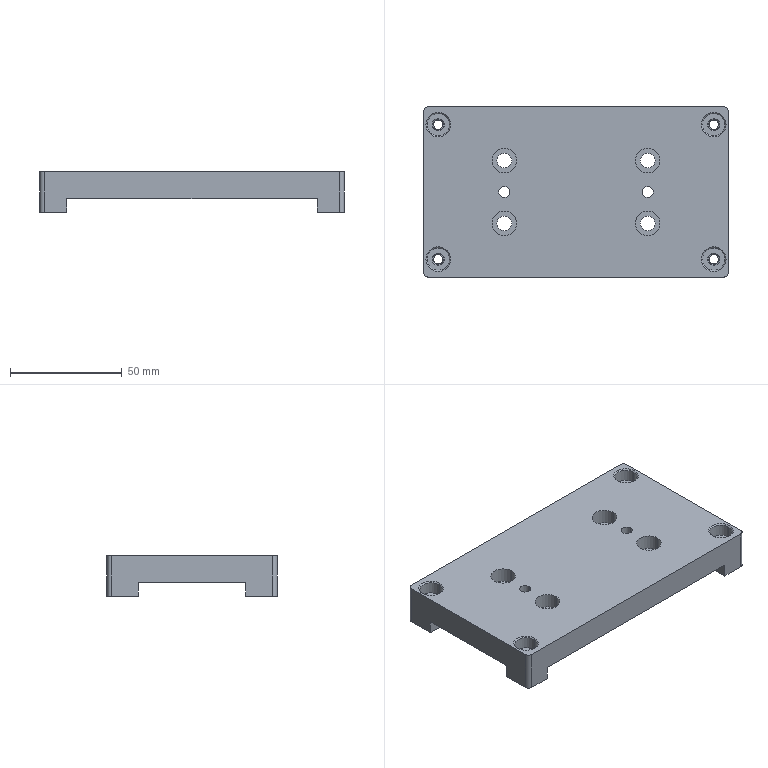Part | STEP file | FBDS-CS-028 | 1 solid | 105 faces | box 136 x 76 x 18 mm | volume 111682 mm3 | cylinder 54 | plane 35 | cone 16 | commonest cylinder face diameters 4 x10 4.2 x8 4.9 x8 6.6 x8 10 x8 11 x8